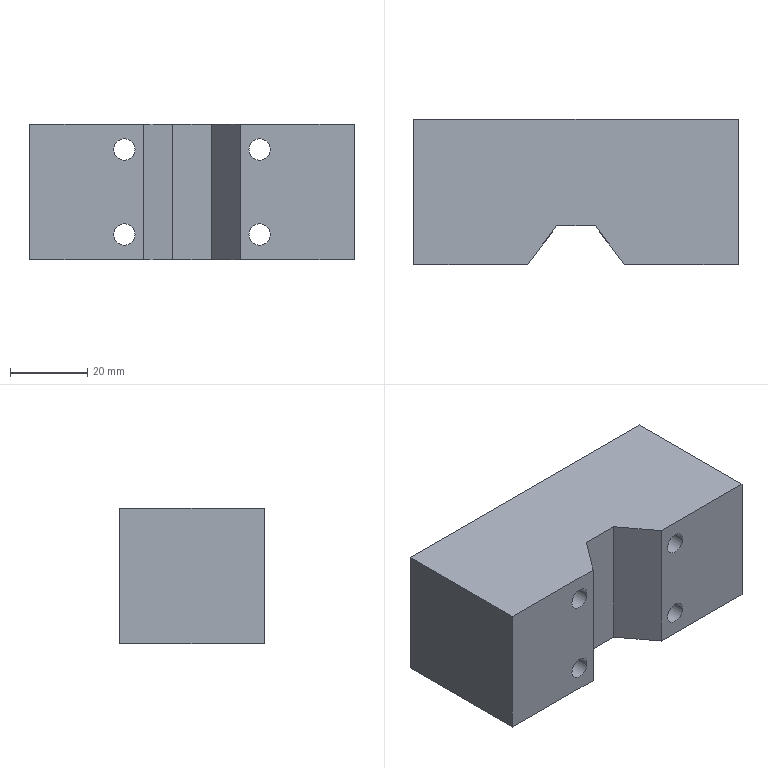Part | NX | features BREP 1 | 1 solid | 46 faces | box 84 x 37.5 x 35 mm | volume 91780 mm3 | cylinder 24 | plane 14 | cone 8 | commonest cylinder face diameters 5.5 x8 6.5 x8 9.5 x8
STEP:
#1=CARTESIAN_POINT('',(-42.,0.,17.5));
#2=VERTEX_POINT('',#1);
#3=CARTESIAN_POINT('',(-12.5,0.,17.5));
#4=VERTEX_POINT('',#3);
#5=CARTESIAN_POINT('',(-42.,0.,17.5));
#6=DIRECTION('',(1.,0.,0.));
#7=VECTOR('',#6,1000.);
#8=LINE('',#5,#7);
#9=EDGE_CURVE('',#2,#4,#8,.T.);
#10=ORIENTED_EDGE('',*,*,#9,.F.);
#11=CARTESIAN_POINT('',(-42.,0.,-17.5));
#12=VERTEX_POINT('',#11);
#13=CARTESIAN_POINT('',(-42.,0.,-17.5));
#14=DIRECTION('',(0.,0.,1.));
#15=VECTOR('',#14,1000.);
#16=LINE('',#13,#15);
#17=EDGE_CURVE('',#12,#2,#16,.T.);
#18=ORIENTED_EDGE('',*,*,#17,.F.);
#19=CARTESIAN_POINT('',(-12.5,0.,-17.5));
#20=VERTEX_POINT('',#19);
#21=CARTESIAN_POINT('',(-12.5,0.,-17.5));
#22=DIRECTION('',(-1.,0.,0.));
#23=VECTOR('',#22,1000.);
#24=LINE('',#21,#23);
#25=EDGE_CURVE('',#20,#12,#24,.T.);
#26=ORIENTED_EDGE('',*,*,#25,.F.);
#27=CARTESIAN_POINT('',(-12.5,0.,17.5));
#28=DIRECTION('',(0.,0.,-1.));
#29=VECTOR('',#28,1000.);
#30=LINE('',#27,#29);
#31=EDGE_CURVE('',#4,#20,#30,.T.);
#32=ORIENTED_EDGE('',*,*,#31,.F.);
#33=EDGE_LOOP('',(#10,#18,#26,#32));
#34=FACE_BOUND('',#33,.T.);
#35=CARTESIAN_POINT('',(-20.25,0.,-11.));
#36=VERTEX_POINT('',#35);
#37=CARTESIAN_POINT('',(-14.75,0.,-11.));
#38=VERTEX_POINT('',#37);
#39=CARTESIAN_POINT('',(-17.5,0.,-11.));
#40=DIRECTION('',(0.,1.,0.));
#41=DIRECTION('',(-1.,0.,0.));
#42=AXIS2_PLACEMENT_3D('',#39,#40,#41);
#43=CIRCLE('',#42,2.75);
#44=EDGE_CURVE('',#36,#38,#43,.T.);
#45=ORIENTED_EDGE('',*,*,#44,.T.);
#46=CARTESIAN_POINT('',(-17.5,0.,-11.));
#47=DIRECTION('',(0.,1.,0.));
#48=DIRECTION('',(1.,0.,0.));
#49=AXIS2_PLACEMENT_3D('',#46,#47,#48);
#50=CIRCLE('',#49,2.75);
#51=EDGE_CURVE('',#38,#36,#50,.T.);
#52=ORIENTED_EDGE('',*,*,#51,.T.);
#53=EDGE_LOOP('',(#45,#52));
#54=FACE_BOUND('',#53,.T.);
#55=CARTESIAN_POINT('',(-20.25,0.,11.));
#56=VERTEX_POINT('',#55);
#57=CARTESIAN_POINT('',(-14.75,0.,11.));
#58=VERTEX_POINT('',#57);
#59=CARTESIAN_POINT('',(-17.5,0.,11.));
#60=DIRECTION('',(0.,1.,0.));
#61=DIRECTION('',(-1.,0.,0.));
#62=AXIS2_PLACEMENT_3D('',#59,#60,#61);
#63=CIRCLE('',#62,2.75);
#64=EDGE_CURVE('',#56,#58,#63,.T.);
#65=ORIENTED_EDGE('',*,*,#64,.T.);
#66=CARTESIAN_POINT('',(-17.5,0.,11.));
#67=DIRECTION('',(0.,1.,0.));
#68=DIRECTION('',(1.,0.,0.));
#69=AXIS2_PLACEMENT_3D('',#66,#67,#68);
#70=CIRCLE('',#69,2.75);
#71=EDGE_CURVE('',#58,#56,#70,.T.);
#72=ORIENTED_EDGE('',*,*,#71,.T.);
#73=EDGE_LOOP('',(#65,#72));
#74=FACE_BOUND('',#73,.T.);
#75=CARTESIAN_POINT('',(0.,0.,0.));
#76=DIRECTION('',(0.,1.,0.));
#77=DIRECTION('',(1.,0.,0.));
#78=AXIS2_PLACEMENT_3D('',#75,#76,#77);
#79=PLANE('',#78);
#80=ADVANCED_FACE('',(#34,#54,#74),#79,.F.);
#81=CARTESIAN_POINT('',(42.,0.,-17.5));
#82=VERTEX_POINT('',#81);
#83=CARTESIAN_POINT('',(12.5,0.,-17.5));
#84=VERTEX_POINT('',#83);
#85=CARTESIAN_POINT('',(42.,0.,-17.5));
#86=DIRECTION('',(-1.,0.,0.));
#87=VECTOR('',#86,1000.);
#88=LINE('',#85,#87);
#89=EDGE_CURVE('',#82,#84,#88,.T.);
#90=ORIENTED_EDGE('',*,*,#89,.F.);
#91=CARTESIAN_POINT('',(42.,0.,17.5));
#92=VERTEX_POINT('',#91);
#93=CARTESIAN_POINT('',(42.,0.,17.5));
#94=DIRECTION('',(0.,0.,-1.));
#95=VECTOR('',#94,1000.);
#96=LINE('',#93,#95);
#97=EDGE_CURVE('',#92,#82,#96,.T.);
#98=ORIENTED_EDGE('',*,*,#97,.F.);
#99=CARTESIAN_POINT('',(12.5,0.,17.5));
#100=VERTEX_POINT('',#99);
#101=CARTESIAN_POINT('',(12.5,0.,17.5));
#102=DIRECTION('',(1.,0.,0.));
#103=VECTOR('',#102,1000.);
#104=LINE('',#101,#103);
#105=EDGE_CURVE('',#100,#92,#104,.T.);
#106=ORIENTED_EDGE('',*,*,#105,.F.);
#107=CARTESIAN_POINT('',(12.5,0.,17.5));
#108=DIRECTION('',(0.,0.,-1.));
#109=VECTOR('',#108,1000.);
#110=LINE('',#107,#109);
#111=EDGE_CURVE('',#100,#84,#110,.T.);
#112=ORIENTED_EDGE('',*,*,#111,.T.);
#113=EDGE_LOOP('',(#90,#98,#106,#112));
#114=FACE_BOUND('',#113,.T.);
#115=CARTESIAN_POINT('',(14.75,0.,-11.));
#116=VERTEX_POINT('',#115);
#117=CARTESIAN_POINT('',(20.25,0.,-11.));
#118=VERTEX_POINT('',#117);
#119=CARTESIAN_POINT('',(17.5,0.,-11.));
#120=DIRECTION('',(0.,1.,0.));
#121=DIRECTION('',(-1.,0.,0.));
#122=AXIS2_PLACEMENT_3D('',#119,#120,#121);
#123=CIRCLE('',#122,2.75);
#124=EDGE_CURVE('',#116,#118,#123,.T.);
#125=ORIENTED_EDGE('',*,*,#124,.T.);
#126=CARTESIAN_POINT('',(17.5,0.,-11.));
#127=DIRECTION('',(0.,1.,0.));
#128=DIRECTION('',(1.,0.,0.));
#129=AXIS2_PLACEMENT_3D('',#126,#127,#128);
#130=CIRCLE('',#129,2.75);
#131=EDGE_CURVE('',#118,#116,#130,.T.);
#132=ORIENTED_EDGE('',*,*,#131,.T.);
#133=EDGE_LOOP('',(#125,#132));
#134=FACE_BOUND('',#133,.T.);
#135=CARTESIAN_POINT('',(14.75,0.,11.));
#136=VERTEX_POINT('',#135);
#137=CARTESIAN_POINT('',(20.25,0.,11.));
#138=VERTEX_POINT('',#137);
#139=CARTESIAN_POINT('',(17.5,0.,11.));
#140=DIRECTION('',(0.,1.,0.));
#141=DIRECTION('',(-1.,0.,0.));
#142=AXIS2_PLACEMENT_3D('',#139,#140,#141);
#143=CIRCLE('',#142,2.75);
#144=EDGE_CURVE('',#136,#138,#143,.T.);
#145=ORIENTED_EDGE('',*,*,#144,.T.);
#146=CARTESIAN_POINT('',(17.5,0.,11.));
#147=DIRECTION('',(0.,1.,0.));
#148=DIRECTION('',(1.,0.,0.));
#149=AXIS2_PLACEMENT_3D('',#146,#147,#148);
#150=CIRCLE('',#149,2.75);
#151=EDGE_CURVE('',#138,#136,#150,.T.);
#152=ORIENTED_EDGE('',*,*,#151,.T.);
#153=EDGE_LOOP('',(#145,#152));
#154=FACE_BOUND('',#153,.T.);
#155=CARTESIAN_POINT('',(0.,0.,0.));
#156=DIRECTION('',(0.,1.,0.));
#157=DIRECTION('',(1.,0.,0.));
#158=AXIS2_PLACEMENT_3D('',#155,#156,#157);
#159=PLANE('',#158);
#160=ADVANCED_FACE('',(#114,#134,#154),#159,.F.);
#161=CARTESIAN_POINT('',(-14.75,12.5,-11.));
#162=VERTEX_POINT('',#161);
#163=CARTESIAN_POINT('',(-14.75,0.,-11.));
#164=DIRECTION('',(0.,1.,0.));
#165=VECTOR('',#164,1000.);
#166=LINE('',#163,#165);
#167=EDGE_CURVE('',#162,#38,#166,.F.);
#168=ORIENTED_EDGE('',*,*,#167,.F.);
#169=CARTESIAN_POINT('',(-20.25,12.5,-11.));
#170=VERTEX_POINT('',#169);
#171=CARTESIAN_POINT('',(-17.5,12.5,-11.));
#172=DIRECTION('',(0.,1.,0.));
#173=DIRECTION('',(1.,0.,0.));
#174=AXIS2_PLACEMENT_3D('',#171,#172,#173);
#175=CIRCLE('',#174,2.75);
#176=EDGE_CURVE('',#162,#170,#175,.T.);
#177=ORIENTED_EDGE('',*,*,#176,.T.);
#178=CARTESIAN_POINT('',(-20.25,0.,-11.));
#179=DIRECTION('',(0.,1.,0.));
#180=VECTOR('',#179,1000.);
#181=LINE('',#178,#180);
#182=EDGE_CURVE('',#170,#36,#181,.F.);
#183=ORIENTED_EDGE('',*,*,#182,.T.);
#184=ORIENTED_EDGE('',*,*,#51,.F.);
#185=EDGE_LOOP('',(#168,#177,#183,#184));
#186=FACE_BOUND('',#185,.T.);
#187=CARTESIAN_POINT('',(-17.5,-16.735,-11.));
#188=DIRECTION('',(0.,1.,0.));
#189=DIRECTION('',(1.,0.,0.));
#190=AXIS2_PLACEMENT_3D('',#187,#188,#189);
#191=CYLINDRICAL_SURFACE('',#190,2.75);
#192=ADVANCED_FACE('',(#186),#191,.F.);
#193=ORIENTED_EDGE('',*,*,#182,.F.);
#194=CARTESIAN_POINT('',(-17.5,12.5,-11.));
#195=DIRECTION('',(0.,-1.,0.));
#196=DIRECTION('',(1.,0.,0.));
#197=AXIS2_PLACEMENT_3D('',#194,#195,#196);
#198=CIRCLE('',#197,2.75);
#199=EDGE_CURVE('',#162,#170,#198,.T.);
#200=ORIENTED_EDGE('',*,*,#199,.F.);
#201=ORIENTED_EDGE('',*,*,#167,.T.);
#202=ORIENTED_EDGE('',*,*,#44,.F.);
#203=EDGE_LOOP('',(#193,#200,#201,#202));
#204=FACE_BOUND('',#203,.T.);
#205=CARTESIAN_POINT('',(-17.5,-16.735,-11.));
#206=DIRECTION('',(0.,1.,0.));
#207=DIRECTION('',(1.,0.,0.));
#208=AXIS2_PLACEMENT_3D('',#205,#206,#207);
#209=CYLINDRICAL_SURFACE('',#208,2.75);
#210=ADVANCED_FACE('',(#204),#209,.F.);
#211=CARTESIAN_POINT('',(-12.75,12.5,-11.));
#212=VERTEX_POINT('',#211);
#213=CARTESIAN_POINT('',(-22.25,12.5,-11.));
#214=VERTEX_POINT('',#213);
#215=CARTESIAN_POINT('',(-17.5,12.5,-11.));
#216=DIRECTION('',(0.,-1.,0.));
#217=DIRECTION('',(1.,0.,0.));
#218=AXIS2_PLACEMENT_3D('',#215,#216,#217);
#219=CIRCLE('',#218,4.75);
#220=EDGE_CURVE('',#212,#214,#219,.T.);
#221=ORIENTED_EDGE('',*,*,#220,.F.);
#222=CARTESIAN_POINT('',(-17.5,12.5,-11.));
#223=DIRECTION('',(0.,1.,0.));
#224=DIRECTION('',(1.,0.,0.));
#225=AXIS2_PLACEMENT_3D('',#222,#223,#224);
#226=CIRCLE('',#225,4.75);
#227=EDGE_CURVE('',#212,#214,#226,.T.);
#228=ORIENTED_EDGE('',*,*,#227,.T.);
#229=EDGE_LOOP('',(#221,#228));
#230=FACE_BOUND('',#229,.T.);
#231=ORIENTED_EDGE('',*,*,#176,.F.);
#232=ORIENTED_EDGE('',*,*,#199,.T.);
#233=EDGE_LOOP('',(#231,#232));
#234=FACE_BOUND('',#233,.T.);
#235=CARTESIAN_POINT('',(-17.5,12.5,-11.));
#236=DIRECTION('',(0.,1.,0.));
#237=DIRECTION('',(1.,0.,0.));
#238=AXIS2_PLACEMENT_3D('',#235,#236,#237);
#239=PLANE('',#238);
#240=ADVANCED_FACE('',(#230,#234),#239,.T.);
#241=CARTESIAN_POINT('',(-22.25,37.5,-11.));
#242=VERTEX_POINT('',#241);
#243=CARTESIAN_POINT('',(-22.25,12.5,-11.));
#244=DIRECTION('',(0.,1.,0.));
#245=VECTOR('',#244,1000.);
#246=LINE('',#243,#245);
#247=EDGE_CURVE('',#214,#242,#246,.T.);
#248=ORIENTED_EDGE('',*,*,#247,.F.);
#249=ORIENTED_EDGE('',*,*,#227,.F.);
#250=CARTESIAN_POINT('',(-12.75,37.5,-11.));
#251=VERTEX_POINT('',#250);
#252=CARTESIAN_POINT('',(-12.75,12.5,-11.));
#253=DIRECTION('',(0.,1.,0.));
#254=VECTOR('',#253,1000.);
#255=LINE('',#252,#254);
#256=EDGE_CURVE('',#212,#251,#255,.T.);
#257=ORIENTED_EDGE('',*,*,#256,.T.);
#258=CARTESIAN_POINT('',(-17.5,37.5,-11.));
#259=DIRECTION('',(0.,1.,0.));
#260=DIRECTION('',(1.,0.,0.));
#261=AXIS2_PLACEMENT_3D('',#258,#259,#260);
#262=CIRCLE('',#261,4.75);
#263=EDGE_CURVE('',#251,#242,#262,.T.);
#264=ORIENTED_EDGE('',*,*,#263,.T.);
#265=EDGE_LOOP('',(#248,#249,#257,#264));
#266=FACE_BOUND('',#265,.T.);
#267=CARTESIAN_POINT('',(-17.5,-16.735,-11.));
#268=DIRECTION('',(0.,1.,0.));
#269=DIRECTION('',(1.,0.,0.));
#270=AXIS2_PLACEMENT_3D('',#267,#268,#269);
#271=CYLINDRICAL_SURFACE('',#270,4.75);
#272=ADVANCED_FACE('',(#266),#271,.F.);
#273=CARTESIAN_POINT('',(42.,37.5,17.5));
#274=VERTEX_POINT('',#273);
#275=CARTESIAN_POINT('',(42.,37.5,-17.5));
#276=VERTEX_POINT('',#275);
#277=CARTESIAN_POINT('',(42.,37.5,17.5));
#278=DIRECTION('',(0.,0.,-1.));
#279=VECTOR('',#278,1000.);
#280=LINE('',#277,#279);
#281=EDGE_CURVE('',#274,#276,#280,.T.);
#282=ORIENTED_EDGE('',*,*,#281,.T.);
#283=CARTESIAN_POINT('',(-42.,37.5,-17.5));
#284=VERTEX_POINT('',#283);
#285=CARTESIAN_POINT('',(42.,37.5,-17.5));
#286=DIRECTION('',(-1.,0.,0.));
#287=VECTOR('',#286,1000.);
#288=LINE('',#285,#287);
#289=EDGE_CURVE('',#276,#284,#288,.T.);
#290=ORIENTED_EDGE('',*,*,#289,.T.);
#291=CARTESIAN_POINT('',(-42.,37.5,17.5));
#292=VERTEX_POINT('',#291);
#293=CARTESIAN_POINT('',(-42.,37.5,-17.5));
#294=DIRECTION('',(0.,0.,1.));
#295=VECTOR('',#294,1000.);
#296=LINE('',#293,#295);
#297=EDGE_CURVE('',#284,#292,#296,.T.);
#298=ORIENTED_EDGE('',*,*,#297,.T.);
#299=CARTESIAN_POINT('',(-42.,37.5,17.5));
#300=DIRECTION('',(1.,0.,0.));
#301=VECTOR('',#300,1000.);
#302=LINE('',#299,#301);
#303=EDGE_CURVE('',#292,#274,#302,.T.);
#304=ORIENTED_EDGE('',*,*,#303,.T.);
#305=EDGE_LOOP('',(#282,#290,#298,#304));
#306=FACE_BOUND('',#305,.T.);
#307=CARTESIAN_POINT('',(-38.75,37.5,-11.));
#308=VERTEX_POINT('',#307);
#309=CARTESIAN_POINT('',(-32.25,37.5,-11.));
#310=VERTEX_POINT('',#309);
#311=CARTESIAN_POINT('',(-35.5,37.5,-11.));
#312=DIRECTION('',(0.,1.,0.));
#313=DIRECTION('',(-1.,0.,0.));
#314=AXIS2_PLACEMENT_3D('',#311,#312,#313);
#315=CIRCLE('',#314,3.25);
#316=EDGE_CURVE('',#308,#310,#315,.T.);
#317=ORIENTED_EDGE('',*,*,#316,.F.);
#318=CARTESIAN_POINT('',(-35.5,37.5,-11.));
#319=DIRECTION('',(0.,1.,0.));
#320=DIRECTION('',(1.,0.,0.));
#321=AXIS2_PLACEMENT_3D('',#318,#319,#320);
#322=CIRCLE('',#321,3.25);
#323=EDGE_CURVE('',#310,#308,#322,.T.);
#324=ORIENTED_EDGE('',*,*,#323,.F.);
#325=EDGE_LOOP('',(#317,#324));
#326=FACE_BOUND('',#325,.T.);
#327=CARTESIAN_POINT('',(35.5,37.5,-14.25));
#328=VERTEX_POINT('',#327);
#329=CARTESIAN_POINT('',(35.5,37.5,-7.75));
#330=VERTEX_POINT('',#329);
#331=CARTESIAN_POINT('',(35.5,37.5,-11.));
#332=DIRECTION('',(0.,1.,0.));
#333=DIRECTION('',(0.,0.,-1.));
#334=AXIS2_PLACEMENT_3D('',#331,#332,#333);
#335=CIRCLE('',#334,3.25);
#336=EDGE_CURVE('',#328,#330,#335,.T.);
#337=ORIENTED_EDGE('',*,*,#336,.F.);
#338=CARTESIAN_POINT('',(35.5,37.5,-11.));
#339=DIRECTION('',(0.,1.,0.));
#340=DIRECTION('',(0.,0.,1.));
#341=AXIS2_PLACEMENT_3D('',#338,#339,#340);
#342=CIRCLE('',#341,3.25);
#343=EDGE_CURVE('',#330,#328,#342,.T.);
#344=ORIENTED_EDGE('',*,*,#343,.F.);
#345=EDGE_LOOP('',(#337,#344));
#346=FACE_BOUND('',#345,.T.);
#347=CARTESIAN_POINT('',(38.75,37.5,11.));
#348=VERTEX_POINT('',#347);
#349=CARTESIAN_POINT('',(32.25,37.5,11.));
#350=VERTEX_POINT('',#349);
#351=CARTESIAN_POINT('',(35.5,37.5,11.));
#352=DIRECTION('',(0.,1.,0.));
#353=DIRECTION('',(1.,0.,0.));
#354=AXIS2_PLACEMENT_3D('',#351,#352,#353);
#355=CIRCLE('',#354,3.25);
#356=EDGE_CURVE('',#348,#350,#355,.T.);
#357=ORIENTED_EDGE('',*,*,#356,.F.);
#358=CARTESIAN_POINT('',(35.5,37.5,11.));
#359=DIRECTION('',(0.,1.,0.));
#360=DIRECTION('',(-1.,0.,0.));
#361=AXIS2_PLACEMENT_3D('',#358,#359,#360);
#362=CIRCLE('',#361,3.25);
#363=EDGE_CURVE('',#350,#348,#362,.T.);
#364=ORIENTED_EDGE('',*,*,#363,.F.);
#365=EDGE_LOOP('',(#357,#364));
#366=FACE_BOUND('',#365,.T.);
#367=CARTESIAN_POINT('',(-32.25,37.5,11.));
#368=VERTEX_POINT('',#367);
#369=CARTESIAN_POINT('',(-38.75,37.5,11.));
#370=VERTEX_POINT('',#369);
#371=CARTESIAN_POINT('',(-35.5,37.5,11.));
#372=DIRECTION('',(0.,1.,0.));
#373=DIRECTION('',(1.,0.,0.));
#374=AXIS2_PLACEMENT_3D('',#371,#372,#373);
#375=CIRCLE('',#374,3.25);
#376=EDGE_CURVE('',#368,#370,#375,.T.);
#377=ORIENTED_EDGE('',*,*,#376,.F.);
#378=CARTESIAN_POINT('',(-35.5,37.5,11.));
#379=DIRECTION('',(0.,1.,0.));
#380=DIRECTION('',(-1.,0.,0.));
#381=AXIS2_PLACEMENT_3D('',#378,#379,#380);
#382=CIRCLE('',#381,3.25);
#383=EDGE_CURVE('',#370,#368,#382,.T.);
#384=ORIENTED_EDGE('',*,*,#383,.F.);
#385=EDGE_LOOP('',(#377,#384));
#386=FACE_BOUND('',#385,.T.);
#387=CARTESIAN_POINT('',(-17.5,37.5,-11.));
#388=DIRECTION('',(0.,1.,0.));
#389=DIRECTION('',(-1.,0.,0.));
#390=AXIS2_PLACEMENT_3D('',#387,#388,#389);
#391=CIRCLE('',#390,4.75);
#392=EDGE_CURVE('',#242,#251,#391,.T.);
#393=ORIENTED_EDGE('',*,*,#392,.F.);
#394=ORIENTED_EDGE('',*,*,#263,.F.);
#395=EDGE_LOOP('',(#393,#394));
#396=FACE_BOUND('',#395,.T.);
#397=CARTESIAN_POINT('',(12.75,37.5,-11.));
#398=VERTEX_POINT('',#397);
#399=CARTESIAN_POINT('',(22.25,37.5,-11.));
#400=VERTEX_POINT('',#399);
#401=CARTESIAN_POINT('',(17.5,37.5,-11.));
#402=DIRECTION('',(0.,1.,0.));
#403=DIRECTION('',(-1.,0.,0.));
#404=AXIS2_PLACEMENT_3D('',#401,#402,#403);
#405=CIRCLE('',#404,4.75);
#406=EDGE_CURVE('',#398,#400,#405,.T.);
#407=ORIENTED_EDGE('',*,*,#406,.F.);
#408=CARTESIAN_POINT('',(17.5,37.5,-11.));
#409=DIRECTION('',(0.,1.,0.));
#410=DIRECTION('',(1.,0.,0.));
#411=AXIS2_PLACEMENT_3D('',#408,#409,#410);
#412=CIRCLE('',#411,4.75);
#413=EDGE_CURVE('',#400,#398,#412,.T.);
#414=ORIENTED_EDGE('',*,*,#413,.F.);
#415=EDGE_LOOP('',(#407,#414));
#416=FACE_BOUND('',#415,.T.);
#417=CARTESIAN_POINT('',(-22.25,37.5,11.));
#418=VERTEX_POINT('',#417);
#419=CARTESIAN_POINT('',(-12.75,37.5,11.));
#420=VERTEX_POINT('',#419);
#421=CARTESIAN_POINT('',(-17.5,37.5,11.));
#422=DIRECTION('',(0.,1.,0.));
#423=DIRECTION('',(-1.,0.,0.));
#424=AXIS2_PLACEMENT_3D('',#421,#422,#423);
#425=CIRCLE('',#424,4.75);
#426=EDGE_CURVE('',#418,#420,#425,.T.);
#427=ORIENTED_EDGE('',*,*,#426,.F.);
#428=CARTESIAN_POINT('',(-17.5,37.5,11.));
#429=DIRECTION('',(0.,1.,0.));
#430=DIRECTION('',(1.,0.,0.));
#431=AXIS2_PLACEMENT_3D('',#428,#429,#430);
#432=CIRCLE('',#431,4.75);
#433=EDGE_CURVE('',#420,#418,#432,.T.);
#434=ORIENTED_EDGE('',*,*,#433,.F.);
#435=EDGE_LOOP('',(#427,#434));
#436=FACE_BOUND('',#435,.T.);
#437=CARTESIAN_POINT('',(12.75,37.5,11.));
#438=VERTEX_POINT('',#437);
#439=CARTESIAN_POINT('',(22.25,37.5,11.));
#440=VERTEX_POINT('',#439);
#441=CARTESIAN_POINT('',(17.5,37.5,11.));
#442=DIRECTION('',(0.,1.,0.));
#443=DIRECTION('',(-1.,0.,0.));
#444=AXIS2_PLACEMENT_3D('',#441,#442,#443);
#445=CIRCLE('',#444,4.75);
#446=EDGE_CURVE('',#438,#440,#445,.T.);
#447=ORIENTED_EDGE('',*,*,#446,.F.);
#448=CARTESIAN_POINT('',(17.5,37.5,11.));
#449=DIRECTION('',(0.,1.,0.));
#450=DIRECTION('',(1.,0.,0.));
#451=AXIS2_PLACEMENT_3D('',#448,#449,#450);
#452=CIRCLE('',#451,4.75);
#453=EDGE_CURVE('',#440,#438,#452,.T.);
#454=ORIENTED_EDGE('',*,*,#453,.F.);
#455=EDGE_LOOP('',(#447,#454));
#456=FACE_BOUND('',#455,.T.);
#457=CARTESIAN_POINT('',(0.,37.5,0.));
#458=DIRECTION('',(0.,1.,0.));
#459=DIRECTION('',(1.,0.,0.));
#460=AXIS2_PLACEMENT_3D('',#457,#458,#459);
#461=PLANE('',#460);
#462=ADVANCED_FACE('',(#306,#326,#346,#366,#386,#396,#416,#436,#456),#461,.T.);
#463=CARTESIAN_POINT('',(-5.,10.,17.5));
#464=VERTEX_POINT('',#463);
#465=CARTESIAN_POINT('',(5.,10.,17.5));
#466=VERTEX_POINT('',#465);
#467=CARTESIAN_POINT('',(-5.,10.,17.5));
#468=DIRECTION('',(1.,0.,0.));
#469=VECTOR('',#468,1000.);
#470=LINE('',#467,#469);
#471=EDGE_CURVE('',#464,#466,#470,.T.);
#472=ORIENTED_EDGE('',*,*,#471,.T.);
#473=CARTESIAN_POINT('',(5.,10.,17.5));
#474=DIRECTION('',(0.6,-0.8,0.));
#475=VECTOR('',#474,1000.);
#476=LINE('',#473,#475);
#477=EDGE_CURVE('',#466,#100,#476,.T.);
#478=ORIENTED_EDGE('',*,*,#477,.T.);
#479=ORIENTED_EDGE('',*,*,#105,.T.);
#480=CARTESIAN_POINT('',(42.,0.,17.5));
#481=DIRECTION('',(0.,1.,0.));
#482=VECTOR('',#481,1000.);
#483=LINE('',#480,#482);
#484=EDGE_CURVE('',#92,#274,#483,.T.);
#485=ORIENTED_EDGE('',*,*,#484,.T.);
#486=ORIENTED_EDGE('',*,*,#303,.F.);
#487=CARTESIAN_POINT('',(-42.,0.,17.5));
#488=DIRECTION('',(0.,1.,0.));
#489=VECTOR('',#488,1000.);
#490=LINE('',#487,#489);
#491=EDGE_CURVE('',#2,#292,#490,.T.);
#492=ORIENTED_EDGE('',*,*,#491,.F.);
#493=ORIENTED_EDGE('',*,*,#9,.T.);
#494=CARTESIAN_POINT('',(-12.5,0.,17.5));
#495=DIRECTION('',(0.6,0.8,0.));
#496=VECTOR('',#495,1000.);
#497=LINE('',#494,#496);
#498=EDGE_CURVE('',#4,#464,#497,.T.);
#499=ORIENTED_EDGE('',*,*,#498,.T.);
#500=EDGE_LOOP('',(#472,#478,#479,#485,#486,#492,#493,#499));
#501=FACE_BOUND('',#500,.T.);
#502=CARTESIAN_POINT('',(-42.,0.,17.5));
#503=DIRECTION('',(0.,0.,1.));
#504=DIRECTION('',(1.,0.,0.));
#505=AXIS2_PLACEMENT_3D('',#502,#503,#504);
#506=PLANE('',#505);
#507=ADVANCED_FACE('',(#501),#506,.T.);
#508=CARTESIAN_POINT('',(-5.,10.,-17.5));
#509=VERTEX_POINT('',#508);
#510=CARTESIAN_POINT('',(-12.5,0.,-17.5));
#511=DIRECTION('',(0.6,0.8,0.));
#512=VECTOR('',#511,1000.);
#513=LINE('',#510,#512);
#514=EDGE_CURVE('',#20,#509,#513,.T.);
#515=ORIENTED_EDGE('',*,*,#514,.T.);
#516=CARTESIAN_POINT('',(-5.,10.,-17.5));
#517=DIRECTION('',(0.,0.,1.));
#518=VECTOR('',#517,1000.);
#519=LINE('',#516,#518);
#520=EDGE_CURVE('',#509,#464,#519,.T.);
#521=ORIENTED_EDGE('',*,*,#520,.T.);
#522=ORIENTED_EDGE('',*,*,#498,.F.);
#523=ORIENTED_EDGE('',*,*,#31,.T.);
#524=EDGE_LOOP('',(#515,#521,#522,#523));
#525=FACE_BOUND('',#524,.T.);
#526=CARTESIAN_POINT('',(-12.5,0.,-17.5));
#527=DIRECTION('',(-0.8,0.6,0.));
#528=DIRECTION('',(0.,0.,1.));
#529=AXIS2_PLACEMENT_3D('',#526,#527,#528);
#530=PLANE('',#529);
#531=ADVANCED_FACE('',(#525),#530,.F.);
#532=ORIENTED_EDGE('',*,*,#520,.F.);
#533=CARTESIAN_POINT('',(5.,10.,-17.5));
#534=VERTEX_POINT('',#533);
#535=CARTESIAN_POINT('',(-5.,10.,-17.5));
#536=DIRECTION('',(1.,0.,0.));
#537=VECTOR('',#536,1000.);
#538=LINE('',#535,#537);
#539=EDGE_CURVE('',#509,#534,#538,.T.);
#540=ORIENTED_EDGE('',*,*,#539,.T.);
#541=CARTESIAN_POINT('',(5.,10.,-17.5));
#542=DIRECTION('',(0.,0.,1.));
#543=VECTOR('',#542,1000.);
#544=LINE('',#541,#543);
#545=EDGE_CURVE('',#534,#466,#544,.T.);
#546=ORIENTED_EDGE('',*,*,#545,.T.);
#547=ORIENTED_EDGE('',*,*,#471,.F.);
#548=EDGE_LOOP('',(#532,#540,#546,#547));
#549=FACE_BOUND('',#548,.T.);
#550=CARTESIAN_POINT('',(-5.,10.,-17.5));
#551=DIRECTION('',(0.,1.,0.));
#552=DIRECTION('',(1.,0.,0.));
#553=AXIS2_PLACEMENT_3D('',#550,#551,#552);
#554=PLANE('',#553);
#555=ADVANCED_FACE('',(#549),#554,.F.);
#556=ORIENTED_EDGE('',*,*,#477,.F.);
#557=ORIENTED_EDGE('',*,*,#545,.F.);
#558=CARTESIAN_POINT('',(5.,10.,-17.5));
#559=DIRECTION('',(0.6,-0.8,0.));
#560=VECTOR('',#559,1000.);
#561=LINE('',#558,#560);
#562=EDGE_CURVE('',#534,#84,#561,.T.);
#563=ORIENTED_EDGE('',*,*,#562,.T.);
#564=ORIENTED_EDGE('',*,*,#111,.F.);
#565=EDGE_LOOP('',(#556,#557,#563,#564));
#566=FACE_BOUND('',#565,.T.);
#567=CARTESIAN_POINT('',(5.,10.,-17.5));
#568=DIRECTION('',(0.8,0.6,0.));
#569=DIRECTION('',(0.,0.,-1.));
#570=AXIS2_PLACEMENT_3D('',#567,#568,#569);
#571=PLANE('',#570);
#572=ADVANCED_FACE('',(#566),#571,.F.);
#573=ORIENTED_EDGE('',*,*,#25,.T.);
#574=CARTESIAN_POINT('',(-42.,0.,-17.5));
#575=DIRECTION('',(0.,1.,0.));
#576=VECTOR('',#575,1000.);
#577=LINE('',#574,#576);
#578=EDGE_CURVE('',#12,#284,#577,.T.);
#579=ORIENTED_EDGE('',*,*,#578,.T.);
#580=ORIENTED_EDGE('',*,*,#289,.F.);
#581=CARTESIAN_POINT('',(42.,0.,-17.5));
#582=DIRECTION('',(0.,1.,0.));
#583=VECTOR('',#582,1000.);
#584=LINE('',#581,#583);
#585=EDGE_CURVE('',#82,#276,#584,.T.);
#586=ORIENTED_EDGE('',*,*,#585,.F.);
#587=ORIENTED_EDGE('',*,*,#89,.T.);
#588=ORIENTED_EDGE('',*,*,#562,.F.);
#589=ORIENTED_EDGE('',*,*,#539,.F.);
#590=ORIENTED_EDGE('',*,*,#514,.F.);
#591=EDGE_LOOP('',(#573,#579,#580,#586,#587,#588,#589,#590));
#592=FACE_BOUND('',#591,.T.);
#593=CARTESIAN_POINT('',(42.,0.,-17.5));
#594=DIRECTION('',(0.,0.,-1.));
#595=DIRECTION('',(0.,-1.,0.));
#596=AXIS2_PLACEMENT_3D('',#593,#594,#595);
#597=PLANE('',#596);
#598=ADVANCED_FACE('',(#592),#597,.T.);
#599=ORIENTED_EDGE('',*,*,#585,.T.);
#600=ORIENTED_EDGE('',*,*,#281,.F.);
#601=ORIENTED_EDGE('',*,*,#484,.F.);
#602=ORIENTED_EDGE('',*,*,#97,.T.);
#603=EDGE_LOOP('',(#599,#600,#601,#602));
#604=FACE_BOUND('',#603,.T.);
#605=CARTESIAN_POINT('',(42.,0.,17.5));
#606=DIRECTION('',(1.,0.,0.));
#607=DIRECTION('',(0.,1.,0.));
#608=AXIS2_PLACEMENT_3D('',#605,#606,#607);
#609=PLANE('',#608);
#610=ADVANCED_FACE('',(#604),#609,.T.);
#611=ORIENTED_EDGE('',*,*,#491,.T.);
#612=ORIENTED_EDGE('',*,*,#297,.F.);
#613=ORIENTED_EDGE('',*,*,#578,.F.);
#614=ORIENTED_EDGE('',*,*,#17,.T.);
#615=EDGE_LOOP('',(#611,#612,#613,#614));
#616=FACE_BOUND('',#615,.T.);
#617=CARTESIAN_POINT('',(-42.,0.,-17.5));
#618=DIRECTION('',(-1.,0.,0.));
#619=DIRECTION('',(0.,0.,1.));
#620=AXIS2_PLACEMENT_3D('',#617,#618,#619);
#621=PLANE('',#620);
#622=ADVANCED_FACE('',(#616),#621,.T.);
#623=CARTESIAN_POINT('',(-38.75,7.5,-11.));
#624=VERTEX_POINT('',#623);
#625=CARTESIAN_POINT('',(-38.75,7.5,-11.));
#626=DIRECTION('',(0.,1.,0.));
#627=VECTOR('',#626,1000.);
#628=LINE('',#625,#627);
#629=EDGE_CURVE('',#624,#308,#628,.T.);
#630=ORIENTED_EDGE('',*,*,#629,.F.);
#631=CARTESIAN_POINT('',(-32.25,7.5,-11.));
#632=VERTEX_POINT('',#631);
#633=CARTESIAN_POINT('',(-35.5,7.5,-11.));
#634=DIRECTION('',(0.,1.,0.));
#635=DIRECTION('',(1.,0.,0.));
#636=AXIS2_PLACEMENT_3D('',#633,#634,#635);
#637=CIRCLE('',#636,3.25);
#638=EDGE_CURVE('',#632,#624,#637,.T.);
#639=ORIENTED_EDGE('',*,*,#638,.F.);
#640=CARTESIAN_POINT('',(-32.25,7.5,-11.));
#641=DIRECTION('',(0.,1.,0.));
#642=VECTOR('',#641,1000.);
#643=LINE('',#640,#642);
#644=EDGE_CURVE('',#632,#310,#643,.T.);
#645=ORIENTED_EDGE('',*,*,#644,.T.);
#646=ORIENTED_EDGE('',*,*,#323,.T.);
#647=EDGE_LOOP('',(#630,#639,#645,#646));
#648=FACE_BOUND('',#647,.T.);
#649=CARTESIAN_POINT('',(-35.5,3.95,-11.));
#650=DIRECTION('',(0.,1.,0.));
#651=DIRECTION('',(1.,0.,0.));
#652=AXIS2_PLACEMENT_3D('',#649,#650,#651);
#653=CYLINDRICAL_SURFACE('',#652,3.25);
#654=ADVANCED_FACE('',(#648),#653,.F.);
#655=ORIENTED_EDGE('',*,*,#644,.F.);
#656=CARTESIAN_POINT('',(-35.5,7.5,-11.));
#657=DIRECTION('',(0.,-1.,0.));
#658=DIRECTION('',(1.,0.,0.));
#659=AXIS2_PLACEMENT_3D('',#656,#657,#658);
#660=CIRCLE('',#659,3.25);
#661=EDGE_CURVE('',#632,#624,#660,.T.);
#662=ORIENTED_EDGE('',*,*,#661,.T.);
#663=ORIENTED_EDGE('',*,*,#629,.T.);
#664=ORIENTED_EDGE('',*,*,#316,.T.);
#665=EDGE_LOOP('',(#655,#662,#663,#664));
#666=FACE_BOUND('',#665,.T.);
#667=CARTESIAN_POINT('',(-35.5,3.95,-11.));
#668=DIRECTION('',(0.,1.,0.));
#669=DIRECTION('',(1.,0.,0.));
#670=AXIS2_PLACEMENT_3D('',#667,#668,#669);
#671=CYLINDRICAL_SURFACE('',#670,3.25);
#672=ADVANCED_FACE('',(#666),#671,.F.);
#673=CARTESIAN_POINT('',(-35.5,5.547,-11.));
#674=VERTEX_POINT('',#673);
#675=CARTESIAN_POINT('',(-35.5,5.547,-11.));
#676=DIRECTION('',(-0.8572,0.515,0.));
#677=VECTOR('',#676,1000.);
#678=LINE('',#675,#677);
#679=EDGE_CURVE('',#624,#674,#678,.F.);
#680=ORIENTED_EDGE('',*,*,#679,.F.);
#681=ORIENTED_EDGE('',*,*,#661,.F.);
#682=CARTESIAN_POINT('',(-35.5,5.547,-11.));
#683=DIRECTION('',(0.8572,0.515,0.));
#684=VECTOR('',#683,1000.);
#685=LINE('',#682,#684);
#686=EDGE_CURVE('',#632,#674,#685,.F.);
#687=ORIENTED_EDGE('',*,*,#686,.T.);
#688=EDGE_LOOP('',(#680,#681,#687));
#689=FACE_BOUND('',#688,.T.);
#690=CARTESIAN_POINT('',(-35.5,6.554,-11.));
#691=DIRECTION('',(0.,1.,0.));
#692=DIRECTION('',(1.,0.,0.));
#693=AXIS2_PLACEMENT_3D('',#690,#691,#692);
#694=CONICAL_SURFACE('',#693,1.676,1.03);
#695=ADVANCED_FACE('',(#689),#694,.F.);
#696=ORIENTED_EDGE('',*,*,#638,.T.);
#697=ORIENTED_EDGE('',*,*,#679,.T.);
#698=ORIENTED_EDGE('',*,*,#686,.F.);
#699=EDGE_LOOP('',(#696,#697,#698));
#700=FACE_BOUND('',#699,.T.);
#701=CARTESIAN_POINT('',(-35.5,6.554,-11.));
#702=DIRECTION('',(0.,1.,0.));
#703=DIRECTION('',(1.,0.,0.));
#704=AXIS2_PLACEMENT_3D('',#701,#702,#703);
#705=CONICAL_SURFACE('',#704,1.676,1.03);
#706=ADVANCED_FACE('',(#700),#705,.F.);
#707=CARTESIAN_POINT('',(35.5,7.5,-14.25));
#708=VERTEX_POINT('',#707);
#709=CARTESIAN_POINT('',(35.5,7.5,-14.25));
#710=DIRECTION('',(0.,1.,0.));
#711=VECTOR('',#710,1000.);
#712=LINE('',#709,#711);
#713=EDGE_CURVE('',#708,#328,#712,.T.);
#714=ORIENTED_EDGE('',*,*,#713,.F.);
#715=CARTESIAN_POINT('',(35.5,7.5,-7.75));
#716=VERTEX_POINT('',#715);
#717=CARTESIAN_POINT('',(35.5,7.5,-11.));
#718=DIRECTION('',(0.,1.,0.));
#719=DIRECTION('',(0.,0.,1.));
#720=AXIS2_PLACEMENT_3D('',#717,#718,#719);
#721=CIRCLE('',#720,3.25);
#722=EDGE_CURVE('',#716,#708,#721,.T.);
#723=ORIENTED_EDGE('',*,*,#722,.F.);
#724=CARTESIAN_POINT('',(35.5,7.5,-7.75));
#725=DIRECTION('',(0.,1.,0.));
#726=VECTOR('',#725,1000.);
#727=LINE('',#724,#726);
#728=EDGE_CURVE('',#716,#330,#727,.T.);
#729=ORIENTED_EDGE('',*,*,#728,.T.);
#730=ORIENTED_EDGE('',*,*,#343,.T.);
#731=EDGE_LOOP('',(#714,#723,#729,#730));
#732=FACE_BOUND('',#731,.T.);
#733=CARTESIAN_POINT('',(35.5,3.95,-11.));
#734=DIRECTION('',(0.,1.,0.));
#735=DIRECTION('',(0.,0.,1.));
#736=AXIS2_PLACEMENT_3D('',#733,#734,#735);
#737=CYLINDRICAL_SURFACE('',#736,3.25);
#738=ADVANCED_FACE('',(#732),#737,.F.);
#739=ORIENTED_EDGE('',*,*,#728,.F.);
#740=CARTESIAN_POINT('',(35.5,7.5,-11.));
#741=DIRECTION('',(0.,-1.,0.));
#742=DIRECTION('',(0.,0.,1.));
#743=AXIS2_PLACEMENT_3D('',#740,#741,#742);
#744=CIRCLE('',#743,3.25);
#745=EDGE_CURVE('',#716,#708,#744,.T.);
#746=ORIENTED_EDGE('',*,*,#745,.T.);
#747=ORIENTED_EDGE('',*,*,#713,.T.);
#748=ORIENTED_EDGE('',*,*,#336,.T.);
#749=EDGE_LOOP('',(#739,#746,#747,#748));
#750=FACE_BOUND('',#749,.T.);
#751=CARTESIAN_POINT('',(35.5,3.95,-11.));
#752=DIRECTION('',(0.,1.,0.));
#753=DIRECTION('',(0.,0.,1.));
#754=AXIS2_PLACEMENT_3D('',#751,#752,#753);
#755=CYLINDRICAL_SURFACE('',#754,3.25);
#756=ADVANCED_FACE('',(#750),#755,.F.);
#757=CARTESIAN_POINT('',(35.5,5.547,-11.));
#758=VERTEX_POINT('',#757);
#759=CARTESIAN_POINT('',(35.5,5.547,-11.));
#760=DIRECTION('',(0.,0.515,-0.8572));
#761=VECTOR('',#760,1000.);
#762=LINE('',#759,#761);
#763=EDGE_CURVE('',#708,#758,#762,.F.);
#764=ORIENTED_EDGE('',*,*,#763,.F.);
#765=ORIENTED_EDGE('',*,*,#745,.F.);
#766=CARTESIAN_POINT('',(35.5,5.547,-11.));
#767=DIRECTION('',(0.,0.515,0.8572));
#768=VECTOR('',#767,1000.);
#769=LINE('',#766,#768);
#770=EDGE_CURVE('',#716,#758,#769,.F.);
#771=ORIENTED_EDGE('',*,*,#770,.T.);
#772=EDGE_LOOP('',(#764,#765,#771));
#773=FACE_BOUND('',#772,.T.);
#774=CARTESIAN_POINT('',(35.5,6.554,-11.));
#775=DIRECTION('',(0.,1.,0.));
#776=DIRECTION('',(0.,0.,1.));
#777=AXIS2_PLACEMENT_3D('',#774,#775,#776);
#778=CONICAL_SURFACE('',#777,1.676,1.03);
#779=ADVANCED_FACE('',(#773),#778,.F.);
#780=ORIENTED_EDGE('',*,*,#722,.T.);
#781=ORIENTED_EDGE('',*,*,#763,.T.);
#782=ORIENTED_EDGE('',*,*,#770,.F.);
#783=EDGE_LOOP('',(#780,#781,#782));
#784=FACE_BOUND('',#783,.T.);
#785=CARTESIAN_POINT('',(35.5,6.554,-11.));
#786=DIRECTION('',(0.,1.,0.));
#787=DIRECTION('',(0.,0.,1.));
#788=AXIS2_PLACEMENT_3D('',#785,#786,#787);
#789=CONICAL_SURFACE('',#788,1.676,1.03);
#790=ADVANCED_FACE('',(#784),#789,.F.);
#791=CARTESIAN_POINT('',(38.75,7.5,11.));
#792=VERTEX_POINT('',#791);
#793=CARTESIAN_POINT('',(38.75,7.5,11.));
#794=DIRECTION('',(0.,1.,0.));
#795=VECTOR('',#794,1000.);
#796=LINE('',#793,#795);
#797=EDGE_CURVE('',#348,#792,#796,.F.);
#798=ORIENTED_EDGE('',*,*,#797,.T.);
#799=CARTESIAN_POINT('',(32.25,7.5,11.));
#800=VERTEX_POINT('',#799);
#801=CARTESIAN_POINT('',(35.5,7.5,11.));
#802=DIRECTION('',(0.,1.,0.));
#803=DIRECTION('',(-1.,0.,0.));
#804=AXIS2_PLACEMENT_3D('',#801,#802,#803);
#805=CIRCLE('',#804,3.25);
#806=EDGE_CURVE('',#800,#792,#805,.T.);
#807=ORIENTED_EDGE('',*,*,#806,.F.);
#808=CARTESIAN_POINT('',(32.25,7.5,11.));
#809=DIRECTION('',(0.,1.,0.));
#810=VECTOR('',#809,1000.);
#811=LINE('',#808,#810);
#812=EDGE_CURVE('',#350,#800,#811,.F.);
#813=ORIENTED_EDGE('',*,*,#812,.F.);
#814=ORIENTED_EDGE('',*,*,#363,.T.);
#815=EDGE_LOOP('',(#798,#807,#813,#814));
#816=FACE_BOUND('',#815,.T.);
#817=CARTESIAN_POINT('',(35.5,3.95,11.));
#818=DIRECTION('',(0.,1.,0.));
#819=DIRECTION('',(-1.,0.,0.));
#820=AXIS2_PLACEMENT_3D('',#817,#818,#819);
#821=CYLINDRICAL_SURFACE('',#820,3.25);
#822=ADVANCED_FACE('',(#816),#821,.F.);
#823=ORIENTED_EDGE('',*,*,#812,.T.);
#824=CARTESIAN_POINT('',(35.5,7.5,11.));
#825=DIRECTION('',(0.,-1.,0.));
#826=DIRECTION('',(-1.,0.,0.));
#827=AXIS2_PLACEMENT_3D('',#824,#825,#826);
#828=CIRCLE('',#827,3.25);
#829=EDGE_CURVE('',#800,#792,#828,.T.);
#830=ORIENTED_EDGE('',*,*,#829,.T.);
#831=ORIENTED_EDGE('',*,*,#797,.F.);
#832=ORIENTED_EDGE('',*,*,#356,.T.);
#833=EDGE_LOOP('',(#823,#830,#831,#832));
#834=FACE_BOUND('',#833,.T.);
#835=CARTESIAN_POINT('',(35.5,3.95,11.));
#836=DIRECTION('',(0.,1.,0.));
#837=DIRECTION('',(-1.,0.,0.));
#838=AXIS2_PLACEMENT_3D('',#835,#836,#837);
#839=CYLINDRICAL_SURFACE('',#838,3.25);
#840=ADVANCED_FACE('',(#834),#839,.F.);
#841=CARTESIAN_POINT('',(35.5,5.547,11.));
#842=VERTEX_POINT('',#841);
#843=CARTESIAN_POINT('',(35.5,5.547,11.));
#844=DIRECTION('',(0.8572,0.515,0.));
#845=VECTOR('',#844,1000.);
#846=LINE('',#843,#845);
#847=EDGE_CURVE('',#842,#792,#846,.T.);
#848=ORIENTED_EDGE('',*,*,#847,.T.);
#849=ORIENTED_EDGE('',*,*,#829,.F.);
#850=CARTESIAN_POINT('',(35.5,5.547,11.));
#851=DIRECTION('',(-0.8572,0.515,0.));
#852=VECTOR('',#851,1000.);
#853=LINE('',#850,#852);
#854=EDGE_CURVE('',#842,#800,#853,.T.);
#855=ORIENTED_EDGE('',*,*,#854,.F.);
#856=EDGE_LOOP('',(#848,#849,#855));
#857=FACE_BOUND('',#856,.T.);
#858=CARTESIAN_POINT('',(35.5,6.554,11.));
#859=DIRECTION('',(0.,1.,0.));
#860=DIRECTION('',(-1.,0.,0.));
#861=AXIS2_PLACEMENT_3D('',#858,#859,#860);
#862=CONICAL_SURFACE('',#861,1.676,1.03);
#863=ADVANCED_FACE('',(#857),#862,.F.);
#864=ORIENTED_EDGE('',*,*,#806,.T.);
#865=ORIENTED_EDGE('',*,*,#847,.F.);
#866=ORIENTED_EDGE('',*,*,#854,.T.);
#867=EDGE_LOOP('',(#864,#865,#866));
#868=FACE_BOUND('',#867,.T.);
#869=CARTESIAN_POINT('',(35.5,6.554,11.));
#870=DIRECTION('',(0.,1.,0.));
#871=DIRECTION('',(-1.,0.,0.));
#872=AXIS2_PLACEMENT_3D('',#869,#870,#871);
#873=CONICAL_SURFACE('',#872,1.676,1.03);
#874=ADVANCED_FACE('',(#868),#873,.F.);
#875=CARTESIAN_POINT('',(-32.25,7.5,11.));
#876=VERTEX_POINT('',#875);
#877=CARTESIAN_POINT('',(-32.25,7.5,11.));
#878=DIRECTION('',(0.,1.,0.));
#879=VECTOR('',#878,1000.);
#880=LINE('',#877,#879);
#881=EDGE_CURVE('',#368,#876,#880,.F.);
#882=ORIENTED_EDGE('',*,*,#881,.T.);
#883=CARTESIAN_POINT('',(-38.75,7.5,11.));
#884=VERTEX_POINT('',#883);
#885=CARTESIAN_POINT('',(-35.5,7.5,11.));
#886=DIRECTION('',(0.,1.,0.));
#887=DIRECTION('',(-1.,0.,0.));
#888=AXIS2_PLACEMENT_3D('',#885,#886,#887);
#889=CIRCLE('',#888,3.25);
#890=EDGE_CURVE('',#884,#876,#889,.T.);
#891=ORIENTED_EDGE('',*,*,#890,.F.);
#892=CARTESIAN_POINT('',(-38.75,7.5,11.));
#893=DIRECTION('',(0.,1.,0.));
#894=VECTOR('',#893,1000.);
#895=LINE('',#892,#894);
#896=EDGE_CURVE('',#370,#884,#895,.F.);
#897=ORIENTED_EDGE('',*,*,#896,.F.);
#898=ORIENTED_EDGE('',*,*,#383,.T.);
#899=EDGE_LOOP('',(#882,#891,#897,#898));
#900=FACE_BOUND('',#899,.T.);
#901=CARTESIAN_POINT('',(-35.5,3.95,11.));
#902=DIRECTION('',(0.,1.,0.));
#903=DIRECTION('',(-1.,0.,0.));
#904=AXIS2_PLACEMENT_3D('',#901,#902,#903);
#905=CYLINDRICAL_SURFACE('',#904,3.25);
#906=ADVANCED_FACE('',(#900),#905,.F.);
#907=ORIENTED_EDGE('',*,*,#896,.T.);
#908=CARTESIAN_POINT('',(-35.5,7.5,11.));
#909=DIRECTION('',(0.,-1.,0.));
#910=DIRECTION('',(-1.,0.,0.));
#911=AXIS2_PLACEMENT_3D('',#908,#909,#910);
#912=CIRCLE('',#911,3.25);
#913=EDGE_CURVE('',#884,#876,#912,.T.);
#914=ORIENTED_EDGE('',*,*,#913,.T.);
#915=ORIENTED_EDGE('',*,*,#881,.F.);
#916=ORIENTED_EDGE('',*,*,#376,.T.);
#917=EDGE_LOOP('',(#907,#914,#915,#916));
#918=FACE_BOUND('',#917,.T.);
#919=CARTESIAN_POINT('',(-35.5,3.95,11.));
#920=DIRECTION('',(0.,1.,0.));
#921=DIRECTION('',(-1.,0.,0.));
#922=AXIS2_PLACEMENT_3D('',#919,#920,#921);
#923=CYLINDRICAL_SURFACE('',#922,3.25);
#924=ADVANCED_FACE('',(#918),#923,.F.);
#925=CARTESIAN_POINT('',(-35.5,5.547,11.));
#926=VERTEX_POINT('',#925);
#927=CARTESIAN_POINT('',(-35.5,5.547,11.));
#928=DIRECTION('',(0.8572,0.515,0.));
#929=VECTOR('',#928,1000.);
#930=LINE('',#927,#929);
#931=EDGE_CURVE('',#926,#876,#930,.T.);
#932=ORIENTED_EDGE('',*,*,#931,.T.);
#933=ORIENTED_EDGE('',*,*,#913,.F.);
#934=CARTESIAN_POINT('',(-35.5,5.547,11.));
#935=DIRECTION('',(-0.8572,0.515,0.));
#936=VECTOR('',#935,1000.);
#937=LINE('',#934,#936);
#938=EDGE_CURVE('',#926,#884,#937,.T.);
#939=ORIENTED_EDGE('',*,*,#938,.F.);
#940=EDGE_LOOP('',(#932,#933,#939));
#941=FACE_BOUND('',#940,.T.);
#942=CARTESIAN_POINT('',(-35.5,6.554,11.));
#943=DIRECTION('',(0.,1.,0.));
#944=DIRECTION('',(-1.,0.,0.));
#945=AXIS2_PLACEMENT_3D('',#942,#943,#944);
#946=CONICAL_SURFACE('',#945,1.676,1.03);
#947=ADVANCED_FACE('',(#941),#946,.F.);
#948=ORIENTED_EDGE('',*,*,#890,.T.);
#949=ORIENTED_EDGE('',*,*,#931,.F.);
#950=ORIENTED_EDGE('',*,*,#938,.T.);
#951=EDGE_LOOP('',(#948,#949,#950));
#952=FACE_BOUND('',#951,.T.);
#953=CARTESIAN_POINT('',(-35.5,6.554,11.));
#954=DIRECTION('',(0.,1.,0.));
#955=DIRECTION('',(-1.,0.,0.));
#956=AXIS2_PLACEMENT_3D('',#953,#954,#955);
#957=CONICAL_SURFACE('',#956,1.676,1.03);
#958=ADVANCED_FACE('',(#952),#957,.F.);
#959=ORIENTED_EDGE('',*,*,#256,.F.);
#960=ORIENTED_EDGE('',*,*,#220,.T.);
#961=ORIENTED_EDGE('',*,*,#247,.T.);
#962=ORIENTED_EDGE('',*,*,#392,.T.);
#963=EDGE_LOOP('',(#959,#960,#961,#962));
#964=FACE_BOUND('',#963,.T.);
#965=CARTESIAN_POINT('',(-17.5,-16.735,-11.));
#966=DIRECTION('',(0.,1.,0.));
#967=DIRECTION('',(1.,0.,0.));
#968=AXIS2_PLACEMENT_3D('',#965,#966,#967);
#969=CYLINDRICAL_SURFACE('',#968,4.75);
#970=ADVANCED_FACE('',(#964),#969,.F.);
#971=CARTESIAN_POINT('',(12.75,12.5,-11.));
#972=VERTEX_POINT('',#971);
#973=CARTESIAN_POINT('',(12.75,12.5,-11.));
#974=DIRECTION('',(0.,1.,0.));
#975=VECTOR('',#974,1000.);
#976=LINE('',#973,#975);
#977=EDGE_CURVE('',#972,#398,#976,.T.);
#978=ORIENTED_EDGE('',*,*,#977,.F.);
#979=CARTESIAN_POINT('',(22.25,12.5,-11.));
#980=VERTEX_POINT('',#979);
#981=CARTESIAN_POINT('',(17.5,12.5,-11.));
#982=DIRECTION('',(0.,1.,0.));
#983=DIRECTION('',(1.,0.,0.));
#984=AXIS2_PLACEMENT_3D('',#981,#982,#983);
#985=CIRCLE('',#984,4.75);
#986=EDGE_CURVE('',#980,#972,#985,.T.);
#987=ORIENTED_EDGE('',*,*,#986,.F.);
#988=CARTESIAN_POINT('',(22.25,12.5,-11.));
#989=DIRECTION('',(0.,1.,0.));
#990=VECTOR('',#989,1000.);
#991=LINE('',#988,#990);
#992=EDGE_CURVE('',#980,#400,#991,.T.);
#993=ORIENTED_EDGE('',*,*,#992,.T.);
#994=ORIENTED_EDGE('',*,*,#413,.T.);
#995=EDGE_LOOP('',(#978,#987,#993,#994));
#996=FACE_BOUND('',#995,.T.);
#997=CARTESIAN_POINT('',(17.5,-16.735,-11.));
#998=DIRECTION('',(0.,1.,0.));
#999=DIRECTION('',(1.,0.,0.));
#1000=AXIS2_PLACEMENT_3D('',#997,#998,#999);
#1001=CYLINDRICAL_SURFACE('',#1000,4.75);
#1002=ADVANCED_FACE('',(#996),#1001,.F.);
#1003=ORIENTED_EDGE('',*,*,#992,.F.);
#1004=CARTESIAN_POINT('',(17.5,12.5,-11.));
#1005=DIRECTION('',(0.,-1.,0.));
#1006=DIRECTION('',(1.,0.,0.));
#1007=AXIS2_PLACEMENT_3D('',#1004,#1005,#1006);
#1008=CIRCLE('',#1007,4.75);
#1009=EDGE_CURVE('',#980,#972,#1008,.T.);
#1010=ORIENTED_EDGE('',*,*,#1009,.T.);
#1011=ORIENTED_EDGE('',*,*,#977,.T.);
#1012=ORIENTED_EDGE('',*,*,#406,.T.);
#1013=EDGE_LOOP('',(#1003,#1010,#1011,#1012));
#1014=FACE_BOUND('',#1013,.T.);
#1015=CARTESIAN_POINT('',(17.5,-16.735,-11.));
#1016=DIRECTION('',(0.,1.,0.));
#1017=DIRECTION('',(1.,0.,0.));
#1018=AXIS2_PLACEMENT_3D('',#1015,#1016,#1017);
#1019=CYLINDRICAL_SURFACE('',#1018,4.75);
#1020=ADVANCED_FACE('',(#1014),#1019,.F.);
#1021=ORIENTED_EDGE('',*,*,#1009,.F.);
#1022=ORIENTED_EDGE('',*,*,#986,.T.);
#1023=EDGE_LOOP('',(#1021,#1022));
#1024=FACE_BOUND('',#1023,.T.);
#1025=CARTESIAN_POINT('',(20.25,12.5,-11.));
#1026=VERTEX_POINT('',#1025);
#1027=CARTESIAN_POINT('',(14.75,12.5,-11.));
#1028=VERTEX_POINT('',#1027);
#1029=CARTESIAN_POINT('',(17.5,12.5,-11.));
#1030=DIRECTION('',(0.,1.,0.));
#1031=DIRECTION('',(1.,0.,0.));
#1032=AXIS2_PLACEMENT_3D('',#1029,#1030,#1031);
#1033=CIRCLE('',#1032,2.75);
#1034=EDGE_CURVE('',#1026,#1028,#1033,.T.);
#1035=ORIENTED_EDGE('',*,*,#1034,.F.);
#1036=CARTESIAN_POINT('',(17.5,12.5,-11.));
#1037=DIRECTION('',(0.,-1.,0.));
#1038=DIRECTION('',(1.,0.,0.));
#1039=AXIS2_PLACEMENT_3D('',#1036,#1037,#1038);
#1040=CIRCLE('',#1039,2.75);
#1041=EDGE_CURVE('',#1026,#1028,#1040,.T.);
#1042=ORIENTED_EDGE('',*,*,#1041,.T.);
#1043=EDGE_LOOP('',(#1035,#1042));
#1044=FACE_BOUND('',#1043,.T.);
#1045=CARTESIAN_POINT('',(17.5,12.5,-11.));
#1046=DIRECTION('',(0.,1.,0.));
#1047=DIRECTION('',(1.,0.,0.));
#1048=AXIS2_PLACEMENT_3D('',#1045,#1046,#1047);
#1049=PLANE('',#1048);
#1050=ADVANCED_FACE('',(#1024,#1044),#1049,.T.);
#1051=CARTESIAN_POINT('',(14.75,0.,-11.));
#1052=DIRECTION('',(0.,1.,0.));
#1053=VECTOR('',#1052,1000.);
#1054=LINE('',#1051,#1053);
#1055=EDGE_CURVE('',#116,#1028,#1054,.T.);
#1056=ORIENTED_EDGE('',*,*,#1055,.T.);
#1057=ORIENTED_EDGE('',*,*,#1041,.F.);
#1058=CARTESIAN_POINT('',(20.25,0.,-11.));
#1059=DIRECTION('',(0.,1.,0.));
#1060=VECTOR('',#1059,1000.);
#1061=LINE('',#1058,#1060);
#1062=EDGE_CURVE('',#118,#1026,#1061,.T.);
#1063=ORIENTED_EDGE('',*,*,#1062,.F.);
#1064=ORIENTED_EDGE('',*,*,#124,.F.);
#1065=EDGE_LOOP('',(#1056,#1057,#1063,#1064));
#1066=FACE_BOUND('',#1065,.T.);
#1067=CARTESIAN_POINT('',(17.5,-16.735,-11.));
#1068=DIRECTION('',(0.,1.,0.));
#1069=DIRECTION('',(1.,0.,0.));
#1070=AXIS2_PLACEMENT_3D('',#1067,#1068,#1069);
#1071=CYLINDRICAL_SURFACE('',#1070,2.75);
#1072=ADVANCED_FACE('',(#1066),#1071,.F.);
#1073=ORIENTED_EDGE('',*,*,#1062,.T.);
#1074=ORIENTED_EDGE('',*,*,#1034,.T.);
#1075=ORIENTED_EDGE('',*,*,#1055,.F.);
#1076=ORIENTED_EDGE('',*,*,#131,.F.);
#1077=EDGE_LOOP('',(#1073,#1074,#1075,#1076));
#1078=FACE_BOUND('',#1077,.T.);
#1079=CARTESIAN_POINT('',(17.5,-16.735,-11.));
#1080=DIRECTION('',(0.,1.,0.));
#1081=DIRECTION('',(1.,0.,0.));
#1082=AXIS2_PLACEMENT_3D('',#1079,#1080,#1081);
#1083=CYLINDRICAL_SURFACE('',#1082,2.75);
#1084=ADVANCED_FACE('',(#1078),#1083,.F.);
#1085=CARTESIAN_POINT('',(-22.25,12.5,11.));
#1086=VERTEX_POINT('',#1085);
#1087=CARTESIAN_POINT('',(-22.25,12.5,11.));
#1088=DIRECTION('',(0.,1.,0.));
#1089=VECTOR('',#1088,1000.);
#1090=LINE('',#1087,#1089);
#1091=EDGE_CURVE('',#1086,#418,#1090,.T.);
#1092=ORIENTED_EDGE('',*,*,#1091,.F.);
#1093=CARTESIAN_POINT('',(-12.75,12.5,11.));
#1094=VERTEX_POINT('',#1093);
#1095=CARTESIAN_POINT('',(-17.5,12.5,11.));
#1096=DIRECTION('',(0.,1.,0.));
#1097=DIRECTION('',(1.,0.,0.));
#1098=AXIS2_PLACEMENT_3D('',#1095,#1096,#1097);
#1099=CIRCLE('',#1098,4.75);
#1100=EDGE_CURVE('',#1094,#1086,#1099,.T.);
#1101=ORIENTED_EDGE('',*,*,#1100,.F.);
#1102=CARTESIAN_POINT('',(-12.75,12.5,11.));
#1103=DIRECTION('',(0.,1.,0.));
#1104=VECTOR('',#1103,1000.);
#1105=LINE('',#1102,#1104);
#1106=EDGE_CURVE('',#1094,#420,#1105,.T.);
#1107=ORIENTED_EDGE('',*,*,#1106,.T.);
#1108=ORIENTED_EDGE('',*,*,#433,.T.);
#1109=EDGE_LOOP('',(#1092,#1101,#1107,#1108));
#1110=FACE_BOUND('',#1109,.T.);
#1111=CARTESIAN_POINT('',(-17.5,-16.735,11.));
#1112=DIRECTION('',(0.,1.,0.));
#1113=DIRECTION('',(1.,0.,0.));
#1114=AXIS2_PLACEMENT_3D('',#1111,#1112,#1113);
#1115=CYLINDRICAL_SURFACE('',#1114,4.75);
#1116=ADVANCED_FACE('',(#1110),#1115,.F.);
#1117=ORIENTED_EDGE('',*,*,#1106,.F.);
#1118=CARTESIAN_POINT('',(-17.5,12.5,11.));
#1119=DIRECTION('',(0.,-1.,0.));
#1120=DIRECTION('',(1.,0.,0.));
#1121=AXIS2_PLACEMENT_3D('',#1118,#1119,#1120);
#1122=CIRCLE('',#1121,4.75);
#1123=EDGE_CURVE('',#1094,#1086,#1122,.T.);
#1124=ORIENTED_EDGE('',*,*,#1123,.T.);
#1125=ORIENTED_EDGE('',*,*,#1091,.T.);
#1126=ORIENTED_EDGE('',*,*,#426,.T.);
#1127=EDGE_LOOP('',(#1117,#1124,#1125,#1126));
#1128=FACE_BOUND('',#1127,.T.);
#1129=CARTESIAN_POINT('',(-17.5,-16.735,11.));
#1130=DIRECTION('',(0.,1.,0.));
#1131=DIRECTION('',(1.,0.,0.));
#1132=AXIS2_PLACEMENT_3D('',#1129,#1130,#1131);
#1133=CYLINDRICAL_SURFACE('',#1132,4.75);
#1134=ADVANCED_FACE('',(#1128),#1133,.F.);
#1135=ORIENTED_EDGE('',*,*,#1123,.F.);
#1136=ORIENTED_EDGE('',*,*,#1100,.T.);
#1137=EDGE_LOOP('',(#1135,#1136));
#1138=FACE_BOUND('',#1137,.T.);
#1139=CARTESIAN_POINT('',(-14.75,12.5,11.));
#1140=VERTEX_POINT('',#1139);
#1141=CARTESIAN_POINT('',(-20.25,12.5,11.));
#1142=VERTEX_POINT('',#1141);
#1143=CARTESIAN_POINT('',(-17.5,12.5,11.));
#1144=DIRECTION('',(0.,1.,0.));
#1145=DIRECTION('',(1.,0.,0.));
#1146=AXIS2_PLACEMENT_3D('',#1143,#1144,#1145);
#1147=CIRCLE('',#1146,2.75);
#1148=EDGE_CURVE('',#1140,#1142,#1147,.T.);
#1149=ORIENTED_EDGE('',*,*,#1148,.F.);
#1150=CARTESIAN_POINT('',(-17.5,12.5,11.));
#1151=DIRECTION('',(0.,-1.,0.));
#1152=DIRECTION('',(1.,0.,0.));
#1153=AXIS2_PLACEMENT_3D('',#1150,#1151,#1152);
#1154=CIRCLE('',#1153,2.75);
#1155=EDGE_CURVE('',#1140,#1142,#1154,.T.);
#1156=ORIENTED_EDGE('',*,*,#1155,.T.);
#1157=EDGE_LOOP('',(#1149,#1156));
#1158=FACE_BOUND('',#1157,.T.);
#1159=CARTESIAN_POINT('',(-17.5,12.5,11.));
#1160=DIRECTION('',(0.,1.,0.));
#1161=DIRECTION('',(1.,0.,0.));
#1162=AXIS2_PLACEMENT_3D('',#1159,#1160,#1161);
#1163=PLANE('',#1162);
#1164=ADVANCED_FACE('',(#1138,#1158),#1163,.T.);
#1165=CARTESIAN_POINT('',(-20.25,0.,11.));
#1166=DIRECTION('',(0.,1.,0.));
#1167=VECTOR('',#1166,1000.);
#1168=LINE('',#1165,#1167);
#1169=EDGE_CURVE('',#56,#1142,#1168,.T.);
#1170=ORIENTED_EDGE('',*,*,#1169,.T.);
#1171=ORIENTED_EDGE('',*,*,#1155,.F.);
#1172=CARTESIAN_POINT('',(-14.75,0.,11.));
#1173=DIRECTION('',(0.,1.,0.));
#1174=VECTOR('',#1173,1000.);
#1175=LINE('',#1172,#1174);
#1176=EDGE_CURVE('',#58,#1140,#1175,.T.);
#1177=ORIENTED_EDGE('',*,*,#1176,.F.);
#1178=ORIENTED_EDGE('',*,*,#64,.F.);
#1179=EDGE_LOOP('',(#1170,#1171,#1177,#1178));
#1180=FACE_BOUND('',#1179,.T.);
#1181=CARTESIAN_POINT('',(-17.5,-16.735,11.));
#1182=DIRECTION('',(0.,1.,0.));
#1183=DIRECTION('',(1.,0.,0.));
#1184=AXIS2_PLACEMENT_3D('',#1181,#1182,#1183);
#1185=CYLINDRICAL_SURFACE('',#1184,2.75);
#1186=ADVANCED_FACE('',(#1180),#1185,.F.);
#1187=ORIENTED_EDGE('',*,*,#1176,.T.);
#1188=ORIENTED_EDGE('',*,*,#1148,.T.);
#1189=ORIENTED_EDGE('',*,*,#1169,.F.);
#1190=ORIENTED_EDGE('',*,*,#71,.F.);
#1191=EDGE_LOOP('',(#1187,#1188,#1189,#1190));
#1192=FACE_BOUND('',#1191,.T.);
#1193=CARTESIAN_POINT('',(-17.5,-16.735,11.));
#1194=DIRECTION('',(0.,1.,0.));
#1195=DIRECTION('',(1.,0.,0.));
#1196=AXIS2_PLACEMENT_3D('',#1193,#1194,#1195);
#1197=CYLINDRICAL_SURFACE('',#1196,2.75);
#1198=ADVANCED_FACE('',(#1192),#1197,.F.);
#1199=CARTESIAN_POINT('',(12.75,12.5,11.));
#1200=VERTEX_POINT('',#1199);
#1201=CARTESIAN_POINT('',(12.75,12.5,11.));
#1202=DIRECTION('',(0.,1.,0.));
#1203=VECTOR('',#1202,1000.);
#1204=LINE('',#1201,#1203);
#1205=EDGE_CURVE('',#1200,#438,#1204,.T.);
#1206=ORIENTED_EDGE('',*,*,#1205,.F.);
#1207=CARTESIAN_POINT('',(22.25,12.5,11.));
#1208=VERTEX_POINT('',#1207);
#1209=CARTESIAN_POINT('',(17.5,12.5,11.));
#1210=DIRECTION('',(0.,1.,0.));
#1211=DIRECTION('',(1.,0.,0.));
#1212=AXIS2_PLACEMENT_3D('',#1209,#1210,#1211);
#1213=CIRCLE('',#1212,4.75);
#1214=EDGE_CURVE('',#1208,#1200,#1213,.T.);
#1215=ORIENTED_EDGE('',*,*,#1214,.F.);
#1216=CARTESIAN_POINT('',(22.25,12.5,11.));
#1217=DIRECTION('',(0.,1.,0.));
#1218=VECTOR('',#1217,1000.);
#1219=LINE('',#1216,#1218);
#1220=EDGE_CURVE('',#1208,#440,#1219,.T.);
#1221=ORIENTED_EDGE('',*,*,#1220,.T.);
#1222=ORIENTED_EDGE('',*,*,#453,.T.);
#1223=EDGE_LOOP('',(#1206,#1215,#1221,#1222));
#1224=FACE_BOUND('',#1223,.T.);
#1225=CARTESIAN_POINT('',(17.5,-16.735,11.));
#1226=DIRECTION('',(0.,1.,0.));
#1227=DIRECTION('',(1.,0.,0.));
#1228=AXIS2_PLACEMENT_3D('',#1225,#1226,#1227);
#1229=CYLINDRICAL_SURFACE('',#1228,4.75);
#1230=ADVANCED_FACE('',(#1224),#1229,.F.);
#1231=ORIENTED_EDGE('',*,*,#1220,.F.);
#1232=CARTESIAN_POINT('',(17.5,12.5,11.));
#1233=DIRECTION('',(0.,-1.,0.));
#1234=DIRECTION('',(1.,0.,0.));
#1235=AXIS2_PLACEMENT_3D('',#1232,#1233,#1234);
#1236=CIRCLE('',#1235,4.75);
#1237=EDGE_CURVE('',#1208,#1200,#1236,.T.);
#1238=ORIENTED_EDGE('',*,*,#1237,.T.);
#1239=ORIENTED_EDGE('',*,*,#1205,.T.);
#1240=ORIENTED_EDGE('',*,*,#446,.T.);
#1241=EDGE_LOOP('',(#1231,#1238,#1239,#1240));
#1242=FACE_BOUND('',#1241,.T.);
#1243=CARTESIAN_POINT('',(17.5,-16.735,11.));
#1244=DIRECTION('',(0.,1.,0.));
#1245=DIRECTION('',(1.,0.,0.));
#1246=AXIS2_PLACEMENT_3D('',#1243,#1244,#1245);
#1247=CYLINDRICAL_SURFACE('',#1246,4.75);
#1248=ADVANCED_FACE('',(#1242),#1247,.F.);
#1249=ORIENTED_EDGE('',*,*,#1237,.F.);
#1250=ORIENTED_EDGE('',*,*,#1214,.T.);
#1251=EDGE_LOOP('',(#1249,#1250));
#1252=FACE_BOUND('',#1251,.T.);
#1253=CARTESIAN_POINT('',(20.25,12.5,11.));
#1254=VERTEX_POINT('',#1253);
#1255=CARTESIAN_POINT('',(14.75,12.5,11.));
#1256=VERTEX_POINT('',#1255);
#1257=CARTESIAN_POINT('',(17.5,12.5,11.));
#1258=DIRECTION('',(0.,1.,0.));
#1259=DIRECTION('',(1.,0.,0.));
#1260=AXIS2_PLACEMENT_3D('',#1257,#1258,#1259);
#1261=CIRCLE('',#1260,2.75);
#1262=EDGE_CURVE('',#1254,#1256,#1261,.T.);
#1263=ORIENTED_EDGE('',*,*,#1262,.F.);
#1264=CARTESIAN_POINT('',(17.5,12.5,11.));
#1265=DIRECTION('',(0.,-1.,0.));
#1266=DIRECTION('',(1.,0.,0.));
#1267=AXIS2_PLACEMENT_3D('',#1264,#1265,#1266);
#1268=CIRCLE('',#1267,2.75);
#1269=EDGE_CURVE('',#1254,#1256,#1268,.T.);
#1270=ORIENTED_EDGE('',*,*,#1269,.T.);
#1271=EDGE_LOOP('',(#1263,#1270));
#1272=FACE_BOUND('',#1271,.T.);
#1273=CARTESIAN_POINT('',(17.5,12.5,11.));
#1274=DIRECTION('',(0.,1.,0.));
#1275=DIRECTION('',(1.,0.,0.));
#1276=AXIS2_PLACEMENT_3D('',#1273,#1274,#1275);
#1277=PLANE('',#1276);
#1278=ADVANCED_FACE('',(#1252,#1272),#1277,.T.);
#1279=CARTESIAN_POINT('',(14.75,0.,11.));
#1280=DIRECTION('',(0.,1.,0.));
#1281=VECTOR('',#1280,1000.);
#1282=LINE('',#1279,#1281);
#1283=EDGE_CURVE('',#136,#1256,#1282,.T.);
#1284=ORIENTED_EDGE('',*,*,#1283,.T.);
#1285=ORIENTED_EDGE('',*,*,#1269,.F.);
#1286=CARTESIAN_POINT('',(20.25,0.,11.));
#1287=DIRECTION('',(0.,1.,0.));
#1288=VECTOR('',#1287,1000.);
#1289=LINE('',#1286,#1288);
#1290=EDGE_CURVE('',#138,#1254,#1289,.T.);
#1291=ORIENTED_EDGE('',*,*,#1290,.F.);
#1292=ORIENTED_EDGE('',*,*,#144,.F.);
#1293=EDGE_LOOP('',(#1284,#1285,#1291,#1292));
#1294=FACE_BOUND('',#1293,.T.);
#1295=CARTESIAN_POINT('',(17.5,-16.735,11.));
#1296=DIRECTION('',(0.,1.,0.));
#1297=DIRECTION('',(1.,0.,0.));
#1298=AXIS2_PLACEMENT_3D('',#1295,#1296,#1297);
#1299=CYLINDRICAL_SURFACE('',#1298,2.75);
#1300=ADVANCED_FACE('',(#1294),#1299,.F.);
#1301=ORIENTED_EDGE('',*,*,#1290,.T.);
#1302=ORIENTED_EDGE('',*,*,#1262,.T.);
#1303=ORIENTED_EDGE('',*,*,#1283,.F.);
#1304=ORIENTED_EDGE('',*,*,#151,.F.);
#1305=EDGE_LOOP('',(#1301,#1302,#1303,#1304));
#1306=FACE_BOUND('',#1305,.T.);
#1307=CARTESIAN_POINT('',(17.5,-16.735,11.));
#1308=DIRECTION('',(0.,1.,0.));
#1309=DIRECTION('',(1.,0.,0.));
#1310=AXIS2_PLACEMENT_3D('',#1307,#1308,#1309);
#1311=CYLINDRICAL_SURFACE('',#1310,2.75);
#1312=ADVANCED_FACE('',(#1306),#1311,.F.);
#1313=CLOSED_SHELL('',(#80,#160,#192,#210,#240,#272,#462,#507,#531,#555,#572,#598,#610,#622,#654,#672,#695,#706,#738,#756,#779,#790,#822,#840,#863,#874,#906,#924,#947,#958,#970,#1002,#1020,#1050,#1072,#1084,#1116,#1134,#1164,#1186,#1198,#1230,#1248,#1278,#1300,#1312));
#1314=MANIFOLD_SOLID_BREP('',#1313);
#1315=(LENGTH_UNIT()NAMED_UNIT(*)SI_UNIT(.MILLI.,.METRE.));
#1316=UNCERTAINTY_MEASURE_WITH_UNIT(LENGTH_MEASURE(0.00001),#1315,'','');
#1317=(NAMED_UNIT(*)PLANE_ANGLE_UNIT()SI_UNIT($,.RADIAN.));
#1318=(NAMED_UNIT(*)SI_UNIT($,.STERADIAN.)SOLID_ANGLE_UNIT());
#1319=(GEOMETRIC_REPRESENTATION_CONTEXT(3)GLOBAL_UNCERTAINTY_ASSIGNED_CONTEXT((#1316))GLOBAL_UNIT_ASSIGNED_CONTEXT((#1315,#1317,#1318))REPRESENTATION_CONTEXT('',''));
#1320=ADVANCED_BREP_SHAPE_REPRESENTATION('',(#1314),#1319);